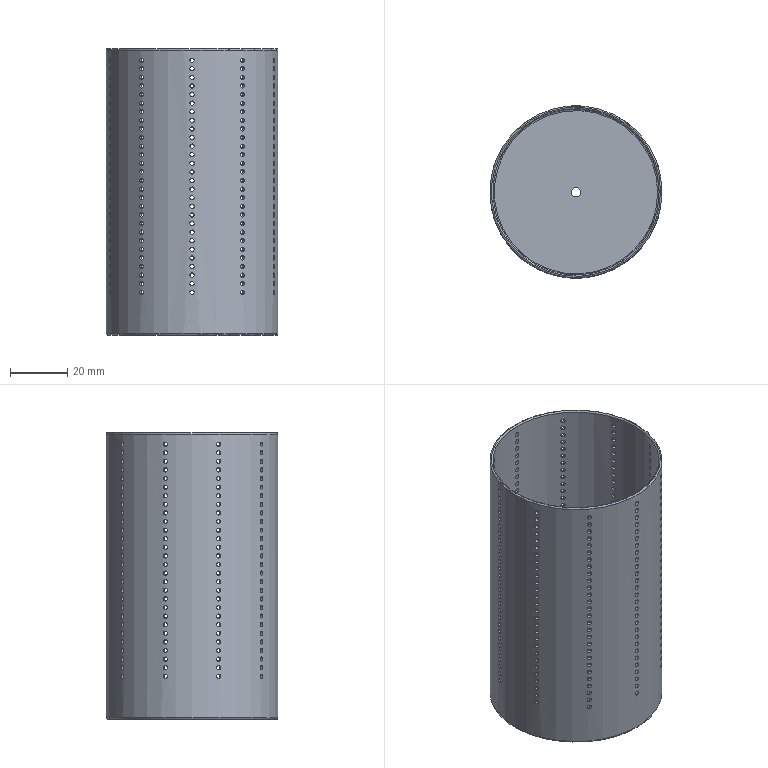Part | STEP file | JBJ-P-1011-02 | 1 solid | 289 faces | box 60 x 60 x 100 mm | volume 25920 mm3 | cylinder 283 | torus 4 | plane 2 | commonest cylinder face diameters 1.5 x280 3.3 x1 58 x1 60 x1